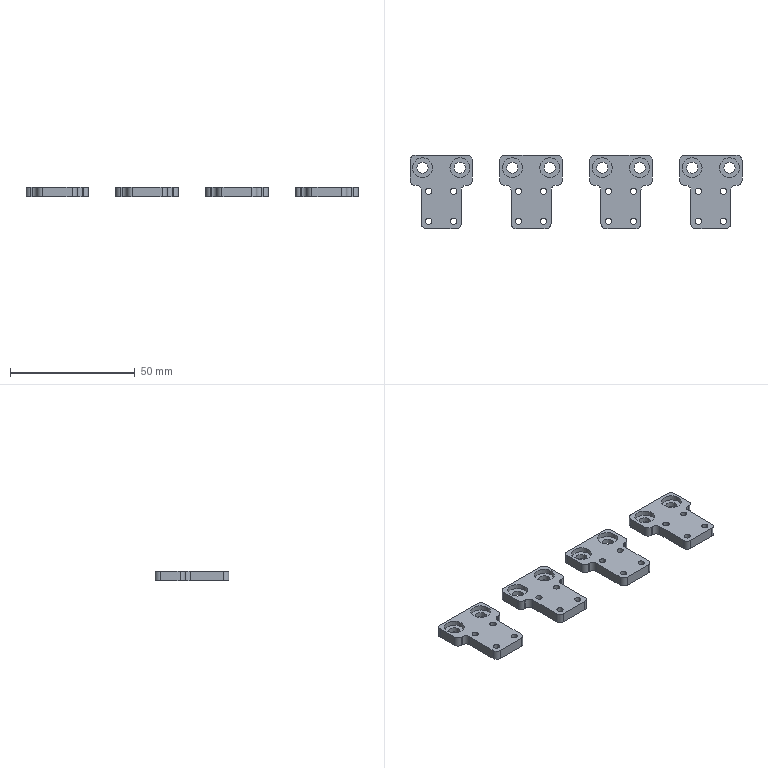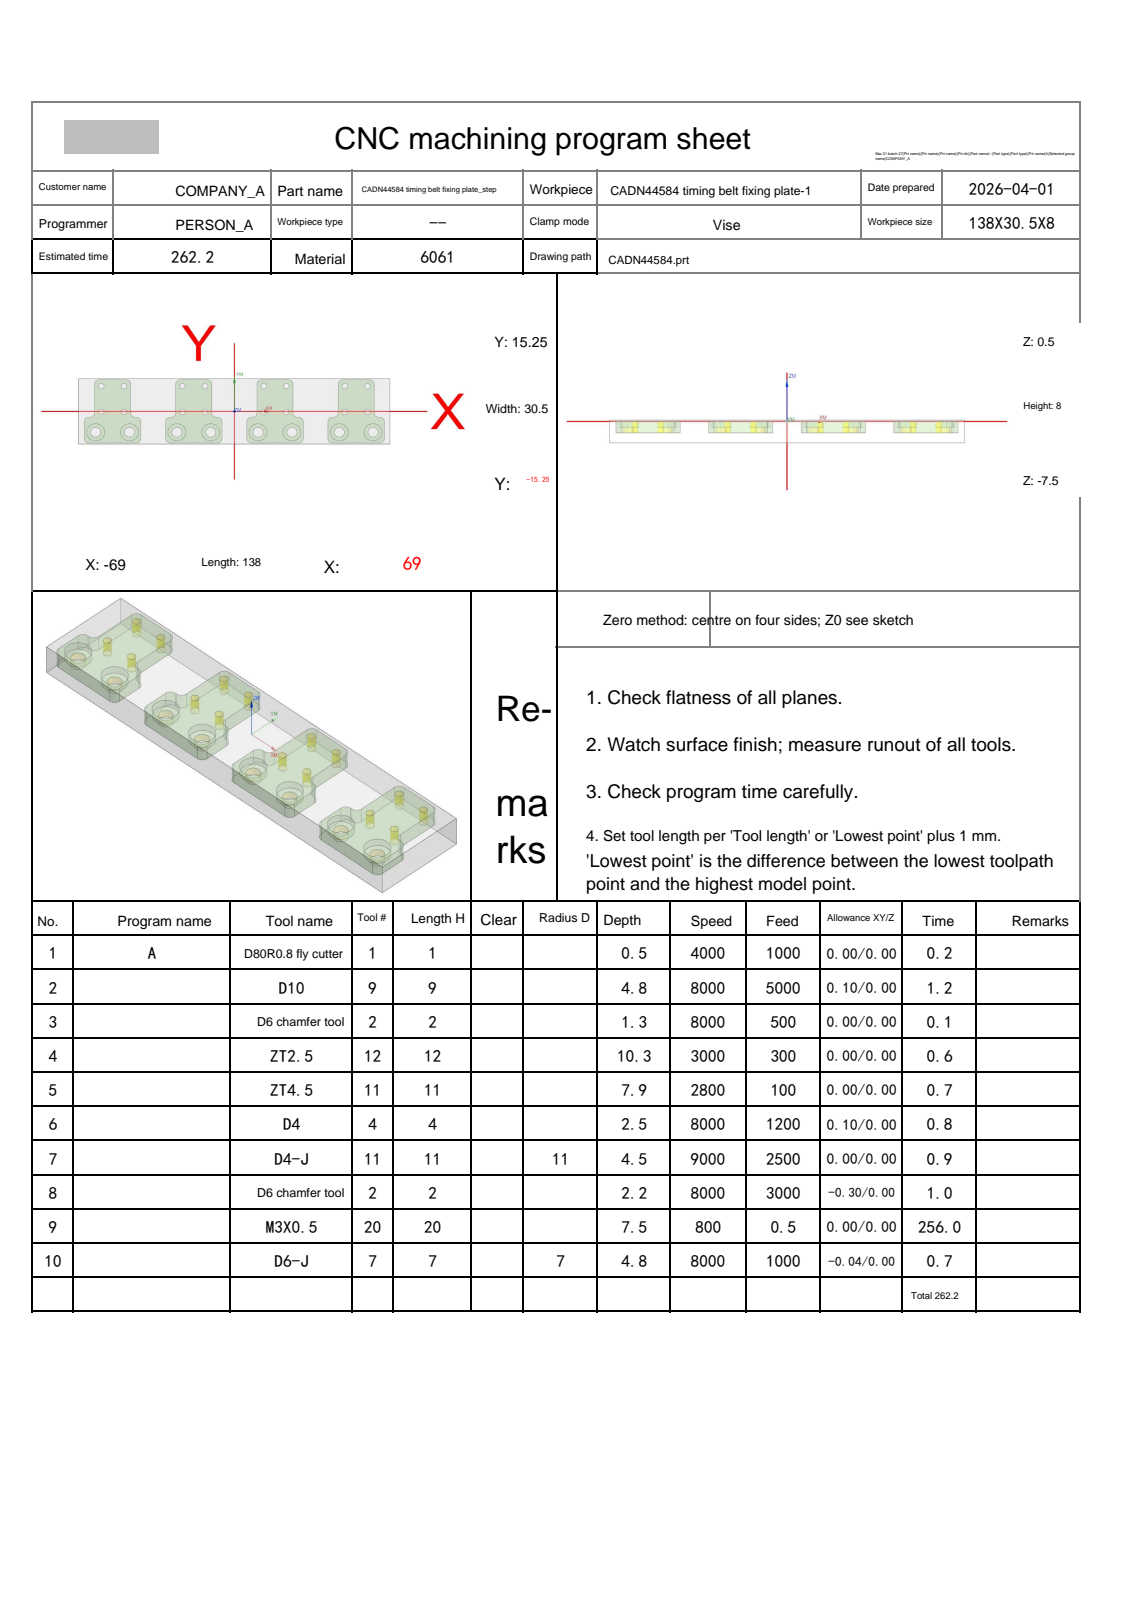NC program | NX | posted by the shop | part box 133 x 29.5 x 4 mm
Lines 1 to 868 of 5056:
%
O0001
(Machine time: 488.18 MIN)
(===Total Tool:8===)
(T1=D80R0.8 fly cutter D=80.  R=0.8  D-  H01 Z=0.    )
(T9=D10     D=10.  R=0.   D-  H09 Z=-4.3  )
(T2=D6 chamfer tool   D=6.   R=0.   D-  H02 Z=-1.75 )
(T12=ZT2.5  D=2.5  DR_a=118 D-  H12 Z=-9.75 )
(T11=ZT4.5  D=4.5  DR_a=118 D-  H11 Z=-7.35 )
(T4=D4      D=4.   R=0.   D-  H04 Z=-2.   )
(T20=M3X0.5 D=2.5  DR_a=180 D-  H20 Z=-7.   )
(T7=D6-J    D=6.   R=0.   D7  H07 Z=-4.3  )
G80 G90 G17 G49 G40
G91 G28 Z0
M01
N1 T01 M06
(D80R0.8 fly cutter  D=80. R=0.8 H=01 ce=0.00 di=0.00)
G00 G90 G54 X111.5 Y0.0 M03 S4000
G43 H01 Z20.
M08
Z2.
G01 Z0.0 F1000.
X106.5
X-106.5
X-111.5
Z2.
G00 Z20.
G91 G28 Z0.0
M05
M09
G91 G28 Z0.0
M01
N2 T09 M06
(D10  D=10. R=0. H=09 ce=0.10 di=0.00)
G00 G90 G54 X-54. Y-19.85 M03 S8000
G43 H09 Z20.
M08
Z.5
G01 X-64.5 Z.462 F5000.
G02 X-71.6 Y-12.75 Z.421 I0.0 J7.1
G01 Y-4.75 Z.392
G02 X-67.1 Y1.857 Z.362 I7.1 J0.0
G01 Y12.75 Z.322
G02 X-60. Y19.85 Z.282 I7.1 J0.0
G01 X-48. Z.238
G02 X-40.9 Y12.75 Z.198 I0.0 J-7.1
G01 Y1.857 Z.158
G02 X-36.4 Y-4.75 Z.128 I-2.6 J-6.607
G01 Y-12.75 Z.099
G02 X-43.5 Y-19.85 Z.058 I-7.1 J0.0
G01 X-64.5 Z-.018
G02 X-71.6 Y-12.75 Z-.059 I0.0 J7.1
G01 Y-4.75 Z-.088
G02 X-67.1 Y1.857 Z-.118 I7.1 J0.0
G01 Y12.75 Z-.158
G02 X-60. Y19.85 Z-.198 I7.1 J0.0
G01 X-48. Z-.242
G02 X-40.9 Y12.75 Z-.282 I0.0 J-7.1
G01 Y1.857 Z-.322
G02 X-36.4 Y-4.75 Z-.352 I-2.6 J-6.607
G01 Y-12.75 Z-.381
G02 X-43.5 Y-19.85 Z-.422 I-7.1 J0.0
G01 X-64.5 Z-.498
G02 X-71.6 Y-12.75 Z-.539 I0.0 J7.1
G01 Y-4.75 Z-.568
G02 X-67.1 Y1.857 Z-.598 I7.1 J0.0
G01 Y12.75 Z-.638
G02 X-60. Y19.85 Z-.678 I7.1 J0.0
G01 X-48. Z-.722
G02 X-40.9 Y12.75 Z-.762 I0.0 J-7.1
G01 Y1.857 Z-.802
G02 X-36.4 Y-4.75 Z-.832 I-2.6 J-6.607
G01 Y-12.75 Z-.861
G02 X-43.5 Y-19.85 Z-.902 I-7.1 J0.0
G01 X-64.5 Z-.978
G02 X-71.6 Y-12.75 Z-1.019 I0.0 J7.1
G01 Y-4.75 Z-1.048
G02 X-67.1 Y1.857 Z-1.078 I7.1 J0.0
G01 Y12.75 Z-1.118
G02 X-60. Y19.85 Z-1.158 I7.1 J0.0
G01 X-48. Z-1.202
G02 X-40.9 Y12.75 Z-1.242 I0.0 J-7.1
G01 Y1.857 Z-1.282
G02 X-36.4 Y-4.75 Z-1.312 I-2.6 J-6.607
G01 Y-12.75 Z-1.341
G02 X-43.5 Y-19.85 Z-1.382 I-7.1 J0.0
G01 X-64.5 Z-1.458
G02 X-71.6 Y-12.75 Z-1.499 I0.0 J7.1
G01 Y-4.75 Z-1.528
G02 X-67.1 Y1.857 Z-1.558 I7.1 J0.0
G01 Y12.75 Z-1.598
G02 X-60. Y19.85 Z-1.638 I7.1 J0.0
G01 X-48. Z-1.682
G02 X-40.9 Y12.75 Z-1.722 I0.0 J-7.1
G01 Y1.857 Z-1.762
G02 X-36.4 Y-4.75 Z-1.792 I-2.6 J-6.607
G01 Y-12.75 Z-1.821
G02 X-43.5 Y-19.85 Z-1.862 I-7.1 J0.0
G01 X-64.5 Z-1.938
G02 X-71.6 Y-12.75 Z-1.979 I0.0 J7.1
G01 Y-4.75 Z-2.008
G02 X-67.1 Y1.857 Z-2.038 I7.1 J0.0
G01 Y12.75 Z-2.078
G02 X-60. Y19.85 Z-2.118 I7.1 J0.0
G01 X-48. Z-2.162
G02 X-40.9 Y12.75 Z-2.202 I0.0 J-7.1
G01 Y1.857 Z-2.242
G02 X-36.4 Y-4.75 Z-2.272 I-2.6 J-6.607
G01 Y-12.75 Z-2.301
G02 X-43.5 Y-19.85 Z-2.342 I-7.1 J0.0
G01 X-64.5 Z-2.418
G02 X-71.6 Y-12.75 Z-2.459 I0.0 J7.1
G01 Y-4.75 Z-2.488
G02 X-67.1 Y1.857 Z-2.518 I7.1 J0.0
G01 Y12.75 Z-2.558
G02 X-60. Y19.85 Z-2.598 I7.1 J0.0
G01 X-48. Z-2.642
G02 X-40.9 Y12.75 Z-2.682 I0.0 J-7.1
G01 Y1.857 Z-2.722
G02 X-36.4 Y-4.75 Z-2.752 I-2.6 J-6.607
G01 Y-12.75 Z-2.781
G02 X-43.5 Y-19.85 Z-2.822 I-7.1 J0.0
G01 X-64.5 Z-2.898
G02 X-71.6 Y-12.75 Z-2.939 I0.0 J7.1
G01 Y-4.75 Z-2.968
G02 X-67.1 Y1.857 Z-2.998 I7.1 J0.0
G01 Y12.75 Z-3.038
G02 X-60. Y19.85 Z-3.078 I7.1 J0.0
G01 X-48. Z-3.122
G02 X-40.9 Y12.75 Z-3.162 I0.0 J-7.1
G01 Y1.857 Z-3.202
G02 X-36.4 Y-4.75 Z-3.232 I-2.6 J-6.607
G01 Y-12.75 Z-3.261
G02 X-43.5 Y-19.85 Z-3.302 I-7.1 J0.0
G01 X-64.5 Z-3.378
G02 X-71.6 Y-12.75 Z-3.419 I0.0 J7.1
G01 Y-4.75 Z-3.448
G02 X-67.1 Y1.857 Z-3.478 I7.1 J0.0
G01 Y12.75 Z-3.518
G02 X-60. Y19.85 Z-3.558 I7.1 J0.0
G01 X-48. Z-3.602
G02 X-40.9 Y12.75 Z-3.642 I0.0 J-7.1
G01 Y1.857 Z-3.682
G02 X-36.4 Y-4.75 Z-3.712 I-2.6 J-6.607
G01 Y-12.75 Z-3.741
G02 X-43.5 Y-19.85 Z-3.782 I-7.1 J0.0
G01 X-64.5 Z-3.858
G02 X-71.6 Y-12.75 Z-3.899 I0.0 J7.1
G01 Y-4.75 Z-3.928
G02 X-67.1 Y1.857 Z-3.958 I7.1 J0.0
G01 Y12.75 Z-3.998
G02 X-60. Y19.85 Z-4.038 I7.1 J0.0
G01 X-48. Z-4.082
G02 X-40.9 Y12.75 Z-4.122 I0.0 J-7.1
G01 Y1.857 Z-4.162
G02 X-36.4 Y-4.75 Z-4.192 I-2.6 J-6.607
G01 Y-12.75 Z-4.221
G02 X-43.5 Y-19.85 Z-4.262 I-7.1 J0.0
G01 X-54. Z-4.3
X-64.5
G02 X-71.6 Y-12.75 I0.0 J7.1
G01 Y-4.75
G02 X-67.1 Y1.857 I7.1 J0.0
G01 Y12.75
G02 X-60. Y19.85 I7.1 J0.0
G01 X-48.
G02 X-40.9 Y12.75 I0.0 J-7.1
G01 Y1.857
G02 X-36.4 Y-4.75 I-2.6 J-6.607
G01 Y-12.75
G02 X-43.5 Y-19.85 I-7.1 J0.0
G01 X-54.
X-54.5
Z-3.3
G00 Z20.
X-18.
Z.5
G01 X-28.5 Z.462
G02 X-35.6 Y-12.75 Z.421 I0.0 J7.1
G01 Y-4.75 Z.392
G02 X-31.1 Y1.857 Z.362 I7.1 J0.0
G01 Y12.75 Z.322
G02 X-24. Y19.85 Z.282 I7.1 J0.0
G01 X-12. Z.238
G02 X-4.9 Y12.75 Z.198 I0.0 J-7.1
G01 Y1.857 Z.158
G02 X-.4 Y-4.75 Z.128 I-2.6 J-6.607
G01 Y-12.75 Z.099
G02 X-7.5 Y-19.85 Z.058 I-7.1 J0.0
G01 X-28.5 Z-.018
G02 X-35.6 Y-12.75 Z-.059 I0.0 J7.1
G01 Y-4.75 Z-.088
G02 X-31.1 Y1.857 Z-.118 I7.1 J0.0
G01 Y12.75 Z-.158
G02 X-24. Y19.85 Z-.198 I7.1 J0.0
G01 X-12. Z-.242
G02 X-4.9 Y12.75 Z-.282 I0.0 J-7.1
G01 Y1.857 Z-.322
G02 X-.4 Y-4.75 Z-.352 I-2.6 J-6.607
G01 Y-12.75 Z-.381
G02 X-7.5 Y-19.85 Z-.422 I-7.1 J0.0
G01 X-28.5 Z-.498
G02 X-35.6 Y-12.75 Z-.539 I0.0 J7.1
G01 Y-4.75 Z-.568
G02 X-31.1 Y1.857 Z-.598 I7.1 J0.0
G01 Y12.75 Z-.638
G02 X-24. Y19.85 Z-.678 I7.1 J0.0
G01 X-12. Z-.722
G02 X-4.9 Y12.75 Z-.762 I0.0 J-7.1
G01 Y1.857 Z-.802
G02 X-.4 Y-4.75 Z-.832 I-2.6 J-6.607
G01 Y-12.75 Z-.861
G02 X-7.5 Y-19.85 Z-.902 I-7.1 J0.0
G01 X-28.5 Z-.978
G02 X-35.6 Y-12.75 Z-1.019 I0.0 J7.1
G01 Y-4.75 Z-1.048
G02 X-31.1 Y1.857 Z-1.078 I7.1 J0.0
G01 Y12.75 Z-1.118
G02 X-24. Y19.85 Z-1.158 I7.1 J0.0
G01 X-12. Z-1.202
G02 X-4.9 Y12.75 Z-1.242 I0.0 J-7.1
G01 Y1.857 Z-1.282
G02 X-.4 Y-4.75 Z-1.312 I-2.6 J-6.607
G01 Y-12.75 Z-1.341
G02 X-7.5 Y-19.85 Z-1.382 I-7.1 J0.0
G01 X-28.5 Z-1.458
G02 X-35.6 Y-12.75 Z-1.499 I0.0 J7.1
G01 Y-4.75 Z-1.528
G02 X-31.1 Y1.857 Z-1.558 I7.1 J0.0
G01 Y12.75 Z-1.598
G02 X-24. Y19.85 Z-1.638 I7.1 J0.0
G01 X-12. Z-1.682
G02 X-4.9 Y12.75 Z-1.722 I0.0 J-7.1
G01 Y1.857 Z-1.762
G02 X-.4 Y-4.75 Z-1.792 I-2.6 J-6.607
G01 Y-12.75 Z-1.821
G02 X-7.5 Y-19.85 Z-1.862 I-7.1 J0.0
G01 X-28.5 Z-1.938
G02 X-35.6 Y-12.75 Z-1.979 I0.0 J7.1
G01 Y-4.75 Z-2.008
G02 X-31.1 Y1.857 Z-2.038 I7.1 J0.0
G01 Y12.75 Z-2.078
G02 X-24. Y19.85 Z-2.118 I7.1 J0.0
G01 X-12. Z-2.162
G02 X-4.9 Y12.75 Z-2.202 I0.0 J-7.1
G01 Y1.857 Z-2.242
G02 X-.4 Y-4.75 Z-2.272 I-2.6 J-6.607
G01 Y-12.75 Z-2.301
G02 X-7.5 Y-19.85 Z-2.342 I-7.1 J0.0
G01 X-28.5 Z-2.418
G02 X-35.6 Y-12.75 Z-2.459 I0.0 J7.1
G01 Y-4.75 Z-2.488
G02 X-31.1 Y1.857 Z-2.518 I7.1 J0.0
G01 Y12.75 Z-2.558
G02 X-24. Y19.85 Z-2.598 I7.1 J0.0
G01 X-12. Z-2.642
G02 X-4.9 Y12.75 Z-2.682 I0.0 J-7.1
G01 Y1.857 Z-2.722
G02 X-.4 Y-4.75 Z-2.752 I-2.6 J-6.607
G01 Y-12.75 Z-2.781
G02 X-7.5 Y-19.85 Z-2.822 I-7.1 J0.0
G01 X-28.5 Z-2.898
G02 X-35.6 Y-12.75 Z-2.939 I0.0 J7.1
G01 Y-4.75 Z-2.968
G02 X-31.1 Y1.857 Z-2.998 I7.1 J0.0
G01 Y12.75 Z-3.038
G02 X-24. Y19.85 Z-3.078 I7.1 J0.0
G01 X-12. Z-3.122
G02 X-4.9 Y12.75 Z-3.162 I0.0 J-7.1
G01 Y1.857 Z-3.202
G02 X-.4 Y-4.75 Z-3.232 I-2.6 J-6.607
G01 Y-12.75 Z-3.261
G02 X-7.5 Y-19.85 Z-3.302 I-7.1 J0.0
G01 X-28.5 Z-3.378
G02 X-35.6 Y-12.75 Z-3.419 I0.0 J7.1
G01 Y-4.75 Z-3.448
G02 X-31.1 Y1.857 Z-3.478 I7.1 J0.0
G01 Y12.75 Z-3.518
G02 X-24. Y19.85 Z-3.558 I7.1 J0.0
G01 X-12. Z-3.602
G02 X-4.9 Y12.75 Z-3.642 I0.0 J-7.1
G01 Y1.857 Z-3.682
G02 X-.4 Y-4.75 Z-3.712 I-2.6 J-6.607
G01 Y-12.75 Z-3.741
G02 X-7.5 Y-19.85 Z-3.782 I-7.1 J0.0
G01 X-28.5 Z-3.858
G02 X-35.6 Y-12.75 Z-3.899 I0.0 J7.1
G01 Y-4.75 Z-3.928
G02 X-31.1 Y1.857 Z-3.958 I7.1 J0.0
G01 Y12.75 Z-3.998
G02 X-24. Y19.85 Z-4.038 I7.1 J0.0
G01 X-12. Z-4.082
G02 X-4.9 Y12.75 Z-4.122 I0.0 J-7.1
G01 Y1.857 Z-4.162
G02 X-.4 Y-4.75 Z-4.192 I-2.6 J-6.607
G01 Y-12.75 Z-4.221
G02 X-7.5 Y-19.85 Z-4.262 I-7.1 J0.0
G01 X-18. Z-4.3
X-28.5
G02 X-35.6 Y-12.75 I0.0 J7.1
G01 Y-4.75
G02 X-31.1 Y1.857 I7.1 J0.0
G01 Y12.75
G02 X-24. Y19.85 I7.1 J0.0
G01 X-12.
G02 X-4.9 Y12.75 I0.0 J-7.1
G01 Y1.857
G02 X-.4 Y-4.75 I-2.6 J-6.607
G01 Y-12.75
G02 X-7.5 Y-19.85 I-7.1 J0.0
G01 X-18.
X-18.5
Z-3.3
G00 Z20.
X18.
Z.5
G01 X7.5 Z.462
G02 X.4 Y-12.75 Z.421 I0.0 J7.1
G01 Y-4.75 Z.392
G02 X4.9 Y1.857 Z.362 I7.1 J0.0
G01 Y12.75 Z.322
G02 X12. Y19.85 Z.282 I7.1 J0.0
G01 X24. Z.238
G02 X31.1 Y12.75 Z.198 I0.0 J-7.1
G01 Y1.857 Z.158
G02 X35.6 Y-4.75 Z.128 I-2.6 J-6.607
G01 Y-12.75 Z.099
G02 X28.5 Y-19.85 Z.058 I-7.1 J0.0
G01 X7.5 Z-.018
G02 X.4 Y-12.75 Z-.059 I0.0 J7.1
G01 Y-4.75 Z-.088
G02 X4.9 Y1.857 Z-.118 I7.1 J0.0
G01 Y12.75 Z-.158
G02 X12. Y19.85 Z-.198 I7.1 J0.0
G01 X24. Z-.242
G02 X31.1 Y12.75 Z-.282 I0.0 J-7.1
G01 Y1.857 Z-.322
G02 X35.6 Y-4.75 Z-.352 I-2.6 J-6.607
G01 Y-12.75 Z-.381
G02 X28.5 Y-19.85 Z-.422 I-7.1 J0.0
G01 X7.5 Z-.498
G02 X.4 Y-12.75 Z-.539 I0.0 J7.1
G01 Y-4.75 Z-.568
G02 X4.9 Y1.857 Z-.598 I7.1 J0.0
G01 Y12.75 Z-.638
G02 X12. Y19.85 Z-.678 I7.1 J0.0
G01 X24. Z-.722
G02 X31.1 Y12.75 Z-.762 I0.0 J-7.1
G01 Y1.857 Z-.802
G02 X35.6 Y-4.75 Z-.832 I-2.6 J-6.607
G01 Y-12.75 Z-.861
G02 X28.5 Y-19.85 Z-.902 I-7.1 J0.0
G01 X7.5 Z-.978
G02 X.4 Y-12.75 Z-1.019 I0.0 J7.1
G01 Y-4.75 Z-1.048
G02 X4.9 Y1.857 Z-1.078 I7.1 J0.0
G01 Y12.75 Z-1.118
G02 X12. Y19.85 Z-1.158 I7.1 J0.0
G01 X24. Z-1.202
G02 X31.1 Y12.75 Z-1.242 I0.0 J-7.1
G01 Y1.857 Z-1.282
G02 X35.6 Y-4.75 Z-1.312 I-2.6 J-6.607
G01 Y-12.75 Z-1.341
G02 X28.5 Y-19.85 Z-1.382 I-7.1 J0.0
G01 X7.5 Z-1.458
G02 X.4 Y-12.75 Z-1.499 I0.0 J7.1
G01 Y-4.75 Z-1.528
G02 X4.9 Y1.857 Z-1.558 I7.1 J0.0
G01 Y12.75 Z-1.598
G02 X12. Y19.85 Z-1.638 I7.1 J0.0
G01 X24. Z-1.682
G02 X31.1 Y12.75 Z-1.722 I0.0 J-7.1
G01 Y1.857 Z-1.762
G02 X35.6 Y-4.75 Z-1.792 I-2.6 J-6.607
G01 Y-12.75 Z-1.821
G02 X28.5 Y-19.85 Z-1.862 I-7.1 J0.0
G01 X7.5 Z-1.938
G02 X.4 Y-12.75 Z-1.979 I0.0 J7.1
G01 Y-4.75 Z-2.008
G02 X4.9 Y1.857 Z-2.038 I7.1 J0.0
G01 Y12.75 Z-2.078
G02 X12. Y19.85 Z-2.118 I7.1 J0.0
G01 X24. Z-2.162
G02 X31.1 Y12.75 Z-2.202 I0.0 J-7.1
G01 Y1.857 Z-2.242
G02 X35.6 Y-4.75 Z-2.272 I-2.6 J-6.607
G01 Y-12.75 Z-2.301
G02 X28.5 Y-19.85 Z-2.342 I-7.1 J0.0
G01 X7.5 Z-2.418
G02 X.4 Y-12.75 Z-2.459 I0.0 J7.1
G01 Y-4.75 Z-2.488
G02 X4.9 Y1.857 Z-2.518 I7.1 J0.0
G01 Y12.75 Z-2.558
G02 X12. Y19.85 Z-2.598 I7.1 J0.0
G01 X24. Z-2.642
G02 X31.1 Y12.75 Z-2.682 I0.0 J-7.1
G01 Y1.857 Z-2.722
G02 X35.6 Y-4.75 Z-2.752 I-2.6 J-6.607
G01 Y-12.75 Z-2.781
G02 X28.5 Y-19.85 Z-2.822 I-7.1 J0.0
G01 X7.5 Z-2.898
G02 X.4 Y-12.75 Z-2.939 I0.0 J7.1
G01 Y-4.75 Z-2.968
G02 X4.9 Y1.857 Z-2.998 I7.1 J0.0
G01 Y12.75 Z-3.038
G02 X12. Y19.85 Z-3.078 I7.1 J0.0
G01 X24. Z-3.122
G02 X31.1 Y12.75 Z-3.162 I0.0 J-7.1
G01 Y1.857 Z-3.202
G02 X35.6 Y-4.75 Z-3.232 I-2.6 J-6.607
G01 Y-12.75 Z-3.261
G02 X28.5 Y-19.85 Z-3.302 I-7.1 J0.0
G01 X7.5 Z-3.378
G02 X.4 Y-12.75 Z-3.419 I0.0 J7.1
G01 Y-4.75 Z-3.448
G02 X4.9 Y1.857 Z-3.478 I7.1 J0.0
G01 Y12.75 Z-3.518
G02 X12. Y19.85 Z-3.558 I7.1 J0.0
G01 X24. Z-3.602
G02 X31.1 Y12.75 Z-3.642 I0.0 J-7.1
G01 Y1.857 Z-3.682
G02 X35.6 Y-4.75 Z-3.712 I-2.6 J-6.607
G01 Y-12.75 Z-3.741
G02 X28.5 Y-19.85 Z-3.782 I-7.1 J0.0
G01 X7.5 Z-3.858
G02 X.4 Y-12.75 Z-3.899 I0.0 J7.1
G01 Y-4.75 Z-3.928
G02 X4.9 Y1.857 Z-3.958 I7.1 J0.0
G01 Y12.75 Z-3.998
G02 X12. Y19.85 Z-4.038 I7.1 J0.0
G01 X24. Z-4.082
G02 X31.1 Y12.75 Z-4.122 I0.0 J-7.1
G01 Y1.857 Z-4.162
G02 X35.6 Y-4.75 Z-4.192 I-2.6 J-6.607
G01 Y-12.75 Z-4.221
G02 X28.5 Y-19.85 Z-4.262 I-7.1 J0.0
G01 X18. Z-4.3
X7.5
G02 X.4 Y-12.75 I0.0 J7.1
G01 Y-4.75
G02 X4.9 Y1.857 I7.1 J0.0
G01 Y12.75
G02 X12. Y19.85 I7.1 J0.0
G01 X24.
G02 X31.1 Y12.75 I0.0 J-7.1
G01 Y1.857
G02 X35.6 Y-4.75 I-2.6 J-6.607
G01 Y-12.75
G02 X28.5 Y-19.85 I-7.1 J0.0
G01 X18.
X17.5
Z-3.3
G00 Z20.
X54.
Z.5
G01 X43.5 Z.462
G02 X36.4 Y-12.75 Z.421 I0.0 J7.1
G01 Y-4.75 Z.392
G02 X40.9 Y1.857 Z.362 I7.1 J0.0
G01 Y12.75 Z.322
G02 X48. Y19.85 Z.282 I7.1 J0.0
G01 X60. Z.238
G02 X67.1 Y12.75 Z.198 I0.0 J-7.1
G01 Y1.857 Z.158
G02 X71.6 Y-4.75 Z.128 I-2.6 J-6.607
G01 Y-12.75 Z.099
G02 X64.5 Y-19.85 Z.058 I-7.1 J0.0
G01 X43.5 Z-.018
G02 X36.4 Y-12.75 Z-.059 I0.0 J7.1
G01 Y-4.75 Z-.088
G02 X40.9 Y1.857 Z-.118 I7.1 J0.0
G01 Y12.75 Z-.158
G02 X48. Y19.85 Z-.198 I7.1 J0.0
G01 X60. Z-.242
G02 X67.1 Y12.75 Z-.282 I0.0 J-7.1
G01 Y1.857 Z-.322
G02 X71.6 Y-4.75 Z-.352 I-2.6 J-6.607
G01 Y-12.75 Z-.381
G02 X64.5 Y-19.85 Z-.422 I-7.1 J0.0
G01 X43.5 Z-.498
G02 X36.4 Y-12.75 Z-.539 I0.0 J7.1
G01 Y-4.75 Z-.568
G02 X40.9 Y1.857 Z-.598 I7.1 J0.0
G01 Y12.75 Z-.638
G02 X48. Y19.85 Z-.678 I7.1 J0.0
G01 X60. Z-.722
G02 X67.1 Y12.75 Z-.762 I0.0 J-7.1
G01 Y1.857 Z-.802
G02 X71.6 Y-4.75 Z-.832 I-2.6 J-6.607
G01 Y-12.75 Z-.861
G02 X64.5 Y-19.85 Z-.902 I-7.1 J0.0
G01 X43.5 Z-.978
G02 X36.4 Y-12.75 Z-1.019 I0.0 J7.1
G01 Y-4.75 Z-1.048
G02 X40.9 Y1.857 Z-1.078 I7.1 J0.0
G01 Y12.75 Z-1.118
G02 X48. Y19.85 Z-1.158 I7.1 J0.0
G01 X60. Z-1.202
G02 X67.1 Y12.75 Z-1.242 I0.0 J-7.1
G01 Y1.857 Z-1.282
G02 X71.6 Y-4.75 Z-1.312 I-2.6 J-6.607
G01 Y-12.75 Z-1.341
G02 X64.5 Y-19.85 Z-1.382 I-7.1 J0.0
G01 X43.5 Z-1.458
G02 X36.4 Y-12.75 Z-1.499 I0.0 J7.1
G01 Y-4.75 Z-1.528
G02 X40.9 Y1.857 Z-1.558 I7.1 J0.0
G01 Y12.75 Z-1.598
G02 X48. Y19.85 Z-1.638 I7.1 J0.0
G01 X60. Z-1.682
G02 X67.1 Y12.75 Z-1.722 I0.0 J-7.1
G01 Y1.857 Z-1.762
G02 X71.6 Y-4.75 Z-1.792 I-2.6 J-6.607
G01 Y-12.75 Z-1.821
G02 X64.5 Y-19.85 Z-1.862 I-7.1 J0.0
G01 X43.5 Z-1.938
G02 X36.4 Y-12.75 Z-1.979 I0.0 J7.1
G01 Y-4.75 Z-2.008
G02 X40.9 Y1.857 Z-2.038 I7.1 J0.0
G01 Y12.75 Z-2.078
G02 X48. Y19.85 Z-2.118 I7.1 J0.0
G01 X60. Z-2.162
G02 X67.1 Y12.75 Z-2.202 I0.0 J-7.1
G01 Y1.857 Z-2.242
G02 X71.6 Y-4.75 Z-2.272 I-2.6 J-6.607
G01 Y-12.75 Z-2.301
G02 X64.5 Y-19.85 Z-2.342 I-7.1 J0.0
G01 X43.5 Z-2.418
G02 X36.4 Y-12.75 Z-2.459 I0.0 J7.1
G01 Y-4.75 Z-2.488
G02 X40.9 Y1.857 Z-2.518 I7.1 J0.0
G01 Y12.75 Z-2.558
G02 X48. Y19.85 Z-2.598 I7.1 J0.0
G01 X60. Z-2.642
G02 X67.1 Y12.75 Z-2.682 I0.0 J-7.1
G01 Y1.857 Z-2.722
G02 X71.6 Y-4.75 Z-2.752 I-2.6 J-6.607
G01 Y-12.75 Z-2.781
G02 X64.5 Y-19.85 Z-2.822 I-7.1 J0.0
G01 X43.5 Z-2.898
G02 X36.4 Y-12.75 Z-2.939 I0.0 J7.1
G01 Y-4.75 Z-2.968
G02 X40.9 Y1.857 Z-2.998 I7.1 J0.0
G01 Y12.75 Z-3.038
G02 X48. Y19.85 Z-3.078 I7.1 J0.0
G01 X60. Z-3.122
G02 X67.1 Y12.75 Z-3.162 I0.0 J-7.1
G01 Y1.857 Z-3.202
G02 X71.6 Y-4.75 Z-3.232 I-2.6 J-6.607
G01 Y-12.75 Z-3.261
G02 X64.5 Y-19.85 Z-3.302 I-7.1 J0.0
G01 X43.5 Z-3.378
G02 X36.4 Y-12.75 Z-3.419 I0.0 J7.1
G01 Y-4.75 Z-3.448
G02 X40.9 Y1.857 Z-3.478 I7.1 J0.0
G01 Y12.75 Z-3.518
G02 X48. Y19.85 Z-3.558 I7.1 J0.0
G01 X60. Z-3.602
G02 X67.1 Y12.75 Z-3.642 I0.0 J-7.1
G01 Y1.857 Z-3.682
G02 X71.6 Y-4.75 Z-3.712 I-2.6 J-6.607
G01 Y-12.75 Z-3.741
G02 X64.5 Y-19.85 Z-3.782 I-7.1 J0.0
G01 X43.5 Z-3.858
G02 X36.4 Y-12.75 Z-3.899 I0.0 J7.1
G01 Y-4.75 Z-3.928
G02 X40.9 Y1.857 Z-3.958 I7.1 J0.0
G01 Y12.75 Z-3.998
G02 X48. Y19.85 Z-4.038 I7.1 J0.0
G01 X60. Z-4.082
G02 X67.1 Y12.75 Z-4.122 I0.0 J-7.1
G01 Y1.857 Z-4.162
G02 X71.6 Y-4.75 Z-4.192 I-2.6 J-6.607
G01 Y-12.75 Z-4.221
G02 X64.5 Y-19.85 Z-4.262 I-7.1 J0.0
G01 X54. Z-4.3
X43.5
G02 X36.4 Y-12.75 I0.0 J7.1
G01 Y-4.75
G02 X40.9 Y1.857 I7.1 J0.0
G01 Y12.75
G02 X48. Y19.85 I7.1 J0.0
G01 X60.
G02 X67.1 Y12.75 I0.0 J-7.1
G01 Y1.857
G02 X71.6 Y-4.75 I-2.6 J-6.607
G01 Y-12.75
G02 X64.5 Y-19.85 I-7.1 J0.0
G01 X54.
X53.5
Z-3.3
G00 Z20.
G91 G28 Z0.0
M05
M09
G91 G28 Z0.0
M01
N3 T02 M06
(D6 chamfer tool  D=6. R=0. H=02 ce=0.00 di=0.00)
G00 G90 G54 X61.5 Y-9.75 M03 S8000
G43 H02 Z20.
M08
G98 G81 X61.5 Y-9.75 Z-.8 R1. F500.
X59. Y-.25
Y11.75
X49.
Y-.25
X46.5 Y-9.75
X25.5
X23. Y-.25
Y11.75
X13.
Y-.25
X10.5 Y-9.75
X-10.5
X-13. Y-.25
Y11.75
X-23.
Y-.25
X-25.5 Y-9.75
X-46.5
X-49. Y-.25
Y11.75
X-59.
Y-.25
X-61.5 Y-9.75
G80
G00 Z20.
G91 G28 Z0.0
M05
M09
G91 G28 Z0.0
M01
N4 T12 M06
(ZT2.5 D=2.5 DR_a=118 H=12)
G00 G90 G54 X49. Y-.25 M03 S3000
G43 H12 Z20.
M08
G98 G83 X49. Y-.25 Z-9.751 R1. F300. Q2.
X59.
Y11.75
X49.
X23.
Y-.25
X13.
Y11.75
X-13.
Y-.25
X-23.
Y11.75
X-49.
X-59.
Y-.25
X-49.
G80
G00 Z20.
G91 G28 Z0.0
M05
M09
G91 G28 Z0.0
M01
N5 T11 M06
(ZT4.5 D=4.5 DR_a=118 H=11)
G00 G90 G54 X-61.5 Y-9.75 M03 S2800
G43 H11 Z20.
M08
G98 G83 X-61.5 Y-9.75 Z-7.352 R1. F100. Q2.
X-46.5
X-25.5
X-10.5
X10.5
X25.5
X46.5
X61.5
G80
G00 Z20.
G91 G28 Z0.0
M05
M09
G91 G28 Z0.0
M01
N6 T04 M06
(D4  D=4. R=0. H=04 ce=0.10 di=0.00)
G00 G90 G54 X-25.5 Y-9.75 M03 S8000
G43 H04 Z20.
M08
Z.5
G03 X-26.45 Y-8.8 I-.95 J0.0 F1200.
X-27.4 Y-9.75 I0.0 J-.95
X-27.4 Y-9.75 Z.2 I1.9 J0.0
X-27.4 Y-9.75 Z-.1 I1.9 J0.0
X-27.4 Y-9.75 Z-.4 I1.9 J0.0
X-27.4 Y-9.75 Z-.7 I1.9 J0.0
X-27.4 Y-9.75 Z-1. I1.9 J0.0
X-27.4 Y-9.75 Z-1.3 I1.9 J0.0
X-27.4 Y-9.75 Z-1.6 I1.9 J0.0
X-27.4 Y-9.75 Z-1.9 I1.9 J0.0
X-24.55 Y-11.395 Z-2. I1.9 J0.0
X-23.6 Y-9.75 I-.95 J1.645
X-25.5 Y-7.85 I-1.9 J0.0
X-27.4 Y-9.75 I0.0 J-1.9
X-25.5 Y-11.65 I1.9 J0.0
X-24.55 Y-11.395 I0.0 J1.9
X-24.075 Y-10.573 I-.475 J.823
X-25.025 Y-9.623 I-.95 J0.0
X-25.5 Y-9.75 I0.0 J-.95
G00 Z20.
X-46.5
Z.5
G03 X-47.45 Y-8.8 I-.95 J0.0
X-48.4 Y-9.75 I0.0 J-.95
X-48.4 Y-9.75 Z.2 I1.9 J0.0
X-48.4 Y-9.75 Z-.1 I1.9 J0.0
X-48.4 Y-9.75 Z-.4 I1.9 J0.0
X-48.4 Y-9.75 Z-.7 I1.9 J0.0
X-48.4 Y-9.75 Z-1. I1.9 J0.0
X-48.4 Y-9.75 Z-1.3 I1.9 J0.0
X-48.4 Y-9.75 Z-1.6 I1.9 J0.0
X-48.4 Y-9.75 Z-1.9 I1.9 J0.0
X-45.55 Y-11.395 Z-2. I1.9 J0.0
X-44.6 Y-9.75 I-.95 J1.645
X-46.5 Y-7.85 I-1.9 J0.0
X-48.4 Y-9.75 I0.0 J-1.9
X-46.5 Y-11.65 I1.9 J0.0
X-45.55 Y-11.395 I0.0 J1.9
X-45.075 Y-10.573 I-.475 J.823
X-46.025 Y-9.623 I-.95 J0.0
X-46.5 Y-9.75 I0.0 J-.95
G00 Z20.
X-61.5
Z.5
G03 X-62.45 Y-8.8 I-.95 J0.0
X-63.4 Y-9.75 I0.0 J-.95
X-63.4 Y-9.75 Z.2 I1.9 J0.0
X-63.4 Y-9.75 Z-.1 I1.9 J0.0
X-63.4 Y-9.75 Z-.4 I1.9 J0.0
X-63.4 Y-9.75 Z-.7 I1.9 J0.0
X-63.4 Y-9.75 Z-1. I1.9 J0.0
X-63.4 Y-9.75 Z-1.3 I1.9 J0.0
X-63.4 Y-9.75 Z-1.6 I1.9 J0.0
X-63.4 Y-9.75 Z-1.9 I1.9 J0.0
X-60.55 Y-11.395 Z-2. I1.9 J0.0
X-59.6 Y-9.75 I-.95 J1.645
X-61.5 Y-7.85 I-1.9 J0.0
X-63.4 Y-9.75 I0.0 J-1.9
X-61.5 Y-11.65 I1.9 J0.0
X-60.55 Y-11.395 I0.0 J1.9
X-60.075 Y-10.573 I-.475 J.823
X-61.025 Y-9.623 I-.95 J0.0
X-61.5 Y-9.75 I0.0 J-.95
G00 Z20.
X-10.5
Z.5
G03 X-11.45 Y-8.8 I-.95 J0.0
X-12.4 Y-9.75 I0.0 J-.95
X-12.4 Y-9.75 Z.2 I1.9 J0.0
X-12.4 Y-9.75 Z-.1 I1.9 J0.0
X-12.4 Y-9.75 Z-.4 I1.9 J0.0
X-12.4 Y-9.75 Z-.7 I1.9 J0.0
X-12.4 Y-9.75 Z-1. I1.9 J0.0
X-12.4 Y-9.75 Z-1.3 I1.9 J0.0
X-12.4 Y-9.75 Z-1.6 I1.9 J0.0
X-12.4 Y-9.75 Z-1.9 I1.9 J0.0
X-9.55 Y-11.395 Z-2. I1.9 J0.0
X-8.6 Y-9.75 I-.95 J1.645
X-10.5 Y-7.85 I-1.9 J0.0
X-12.4 Y-9.75 I0.0 J-1.9
X-10.5 Y-11.65 I1.9 J0.0
X-9.55 Y-11.395 I0.0 J1.9
X-9.075 Y-10.573 I-.475 J.823
X-10.025 Y-9.623 I-.95 J0.0
X-10.5 Y-9.75 I0.0 J-.95
G00 Z20.
X10.5
Z.5
G03 X9.55 Y-8.8 I-.95 J0.0
X8.6 Y-9.75 I0.0 J-.95
X8.6 Y-9.75 Z.2 I1.9 J0.0
X8.6 Y-9.75 Z-.1 I1.9 J0.0
X8.6 Y-9.75 Z-.4 I1.9 J0.0
X8.6 Y-9.75 Z-.7 I1.9 J0.0
X8.6 Y-9.75 Z-1. I1.9 J0.0
X8.6 Y-9.75 Z-1.3 I1.9 J0.0
X8.6 Y-9.75 Z-1.6 I1.9 J0.0
X8.6 Y-9.75 Z-1.9 I1.9 J0.0
X11.45 Y-11.395 Z-2. I1.9 J0.0
X12.4 Y-9.75 I-.95 J1.645
X10.5 Y-7.85 I-1.9 J0.0
X8.6 Y-9.75 I0.0 J-1.9
X10.5 Y-11.65 I1.9 J0.0
X11.45 Y-11.395 I0.0 J1.9
X11.925 Y-10.573 I-.475 J.823
X10.975 Y-9.623 I-.95 J0.0
X10.5 Y-9.75 I0.0 J-.95
G00 Z20.
X25.5
Z.5
G03 X24.55 Y-8.8 I-.95 J0.0
X23.6 Y-9.75 I0.0 J-.95
X23.6 Y-9.75 Z.2 I1.9 J0.0
X23.6 Y-9.75 Z-.1 I1.9 J0.0
X23.6 Y-9.75 Z-.4 I1.9 J0.0
X23.6 Y-9.75 Z-.7 I1.9 J0.0
X23.6 Y-9.75 Z-1. I1.9 J0.0
X23.6 Y-9.75 Z-1.3 I1.9 J0.0
X23.6 Y-9.75 Z-1.6 I1.9 J0.0
X23.6 Y-9.75 Z-1.9 I1.9 J0.0
X26.45 Y-11.395 Z-2. I1.9 J0.0
X27.4 Y-9.75 I-.95 J1.645
X25.5 Y-7.85 I-1.9 J0.0
X23.6 Y-9.75 I0.0 J-1.9
X25.5 Y-11.65 I1.9 J0.0
X26.45 Y-11.395 I0.0 J1.9
X26.925 Y-10.573 I-.475 J.823
X25.975 Y-9.623 I-.95 J0.0
X25.5 Y-9.75 I0.0 J-.95
G00 Z20.
X46.5
Z.5
G03 X45.55 Y-8.8 I-.95 J0.0
X44.6 Y-9.75 I0.0 J-.95
X44.6 Y-9.75 Z.2 I1.9 J0.0
X44.6 Y-9.75 Z-.1 I1.9 J0.0
X44.6 Y-9.75 Z-.4 I1.9 J0.0
X44.6 Y-9.75 Z-.7 I1.9 J0.0
X44.6 Y-9.75 Z-1. I1.9 J0.0
X44.6 Y-9.75 Z-1.3 I1.9 J0.0
X44.6 Y-9.75 Z-1.6 I1.9 J0.0
X44.6 Y-9.75 Z-1.9 I1.9 J0.0
X47.45 Y-11.395 Z-2. I1.9 J0.0
X48.4 Y-9.75 I-.95 J1.645
X46.5 Y-7.85 I-1.9 J0.0
X44.6 Y-9.75 I0.0 J-1.9
X46.5 Y-11.65 I1.9 J0.0
X47.45 Y-11.395 I0.0 J1.9
X47.925 Y-10.573 I-.475 J.823
X46.975 Y-9.623 I-.95 J0.0
X46.5 Y-9.75 I0.0 J-.95
G00 Z20.
X61.5
Z.5
G03 X60.55 Y-8.8 I-.95 J0.0
X59.6 Y-9.75 I0.0 J-.95
X59.6 Y-9.75 Z.2 I1.9 J0.0
X59.6 Y-9.75 Z-.1 I1.9 J0.0
X59.6 Y-9.75 Z-.4 I1.9 J0.0
X59.6 Y-9.75 Z-.7 I1.9 J0.0
X59.6 Y-9.75 Z-1. I1.9 J0.0
X59.6 Y-9.75 Z-1.3 I1.9 J0.0
X59.6 Y-9.75 Z-1.6 I1.9 J0.0
X59.6 Y-9.75 Z-1.9 I1.9 J0.0
X62.45 Y-11.395 Z-2. I1.9 J0.0
X63.4 Y-9.75 I-.95 J1.645
X61.5 Y-7.85 I-1.9 J0.0
X59.6 Y-9.75 I0.0 J-1.9
X61.5 Y-11.65 I1.9 J0.0
X62.45 Y-11.395 I0.0 J1.9
X62.925 Y-10.573 I-.475 J.823
X61.975 Y-9.623 I-.95 J0.0
X61.5 Y-9.75 I0.0 J-.95
G00 Z20.
G91 G28 Z0.0
M05
M09
G91 G28 Z0.0
M01